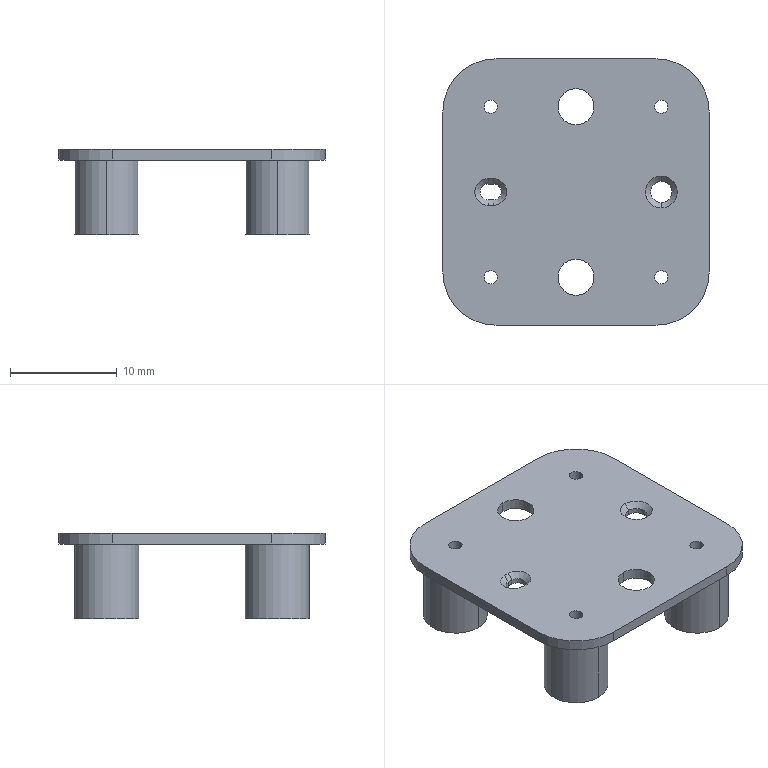NC program | NX | posted with a generic post | part box 25 x 25 x 8 mm
Whole program, first 1563 of 1707 lines:
N10 G17 G21 G94 G90
(FLOOR_WALL_COPY_COPY , TOOL : D80)
N12 T19 M6
N14 G54
N16 G17 G0 G90 X-57.5 Y0. S6500 M3
N18 G43 Z30. H19
N20 Z6.
N22 G94 G1 Z3. F1500.
N24 X-52.5
N26 X52.5
N28 X57.5
N30 Z6.
N32 G0 Z30.
N34 X-57.5
N36 Z5.
N38 G1 Z2.
N40 X-52.5
N42 X52.5
N44 X57.5
N46 Z5.
N48 G0 Z30.
N50 X-57.5
N52 Z4.
N54 G1 Z1.
N56 X-52.5
N58 X52.5
N60 X57.5
N62 Z4.
N64 G0 Z30.
N66 X-57.5
N68 Z3.
N70 G1 Z0.
N72 X-52.5
N74 X52.5
N76 X57.5
N78 Z3.
N80 G0 Z30.
N82 M5
(FLOOR_WALL , TOOL : D4)
N84 T11 M6
N86 G54
N88 G17 G0 G90 X1.026 Y-15.5 S9500 M3
N90 G43 Z30. H11
N92 Z0.617
N94 G94 G1 Z-0.383 F1000.
N96 X0.306 Y-14.643
N98 G3 X0. Y-14.5 R0.4
N100 G1 X-7.5 F2000.
N102 G2 X-14.5 Y-7.5 R7.
N104 G1 Y7.5
N106 G2 X-7.5 Y14.5 R7.
N108 G1 X7.5
N110 G2 X14.5 Y7.5 R7.
N112 G1 Y-7.5
N114 G2 X7.5 Y-14.5 R7.
N116 G1 X0.
N118 Y-12.5
N120 X-4.838
N122 G3 X-12.5 Y-4.838 R-5.5
N124 G1 X-12.173 Y-5.068
N126 G2 X-5.068 Y-3.827 R5.1
N128 X-12.173 Y-5.068 R-5.1
N130 G1 X-12.5 Y-4.838
N132 Y4.838
N134 G3 X-4.838 Y12.5 R-5.5
N136 G1 X-5.068 Y12.173
N138 G2 X-3.827 Y5.068 R5.1
N140 X-5.068 Y12.173 R-5.1
N142 G1 X-4.838 Y12.5
N144 X4.838
N146 G3 X12.5 Y4.838 R-5.5
N148 G1 X12.173 Y5.068
N150 G2 X5.068 Y3.827 R5.1
N152 X12.173 Y5.068 R-5.1
N154 G1 X12.5 Y4.838
N156 Y-4.838
N158 G3 X4.838 Y-12.5 R-5.5
N160 G1 X5.068 Y-12.173
N162 G2 X3.827 Y-5.068 R5.1
N164 X5.068 Y-12.173 R-5.1
N166 G1 X4.838 Y-12.5
N168 X0.
N170 Y-10.5
N172 X-0.929
N174 G3 X-10.5 Y-0.929 R7.5
N176 G1 Y0.929
N178 G3 X-0.929 Y10.5 R7.5
N180 G1 X0.929
N182 G3 X10.5 Y0.929 R7.5
N184 G1 Y-0.929
N186 G3 X1.684 Y-3.955 R7.5
N188 G1 X0. Y-2.877
N190 G3 X-2.877 Y0. R9.5
N192 X0. Y2.877 R9.5
N194 X2.877 Y0. R9.5
N196 X0. Y-2.877 R9.5
N198 G1 Y-0.019
N200 X-0.019 Y0.
N202 X0. Y0.019
N204 X0.019 Y0.
N206 X0. Y-0.019
N208 Y-2.877
N210 X1.684 Y-3.955
N212 G3 X0.929 Y-10.5 R7.5
N214 G1 X0.
N216 G3 X-0.306 Y-10.643 R0.4
N218 G1 Z0.617
N220 G0 X1.026 Y-15.5 Z0.233
N222 G1 Z-0.767 F1000.
N224 X0.306 Y-14.643
N226 G3 X0. Y-14.5 R0.4
N228 G1 X-7.5 F2000.
N230 G2 X-14.5 Y-7.5 R7.
N232 G1 Y7.5
N234 G2 X-7.5 Y14.5 R7.
N236 G1 X7.5
N238 G2 X14.5 Y7.5 R7.
N240 G1 Y-7.5
N242 G2 X7.5 Y-14.5 R7.
N244 G1 X0.
N246 Y-12.5
N248 X-4.838
N250 G3 X-12.5 Y-4.838 R-5.5
N252 G1 X-12.173 Y-5.068
N254 G2 X-5.068 Y-3.827 R5.1
N256 X-12.173 Y-5.068 R-5.1
N258 G1 X-12.5 Y-4.838
N260 Y4.838
N262 G3 X-4.838 Y12.5 R-5.5
N264 G1 X-5.068 Y12.173
N266 G2 X-3.827 Y5.068 R5.1
N268 X-5.068 Y12.173 R-5.1
N270 G1 X-4.838 Y12.5
N272 X4.838
N274 G3 X12.5 Y4.838 R-5.5
N276 G1 X12.173 Y5.068
N278 G2 X5.068 Y3.827 R5.1
N280 X12.173 Y5.068 R-5.1
N282 G1 X12.5 Y4.838
N284 Y-4.838
N286 G3 X4.838 Y-12.5 R-5.5
N288 G1 X5.068 Y-12.173
N290 G2 X3.827 Y-5.068 R5.1
N292 X5.068 Y-12.173 R-5.1
N294 G1 X4.838 Y-12.5
N296 X0.
N298 Y-10.5
N300 X-0.929
N302 G3 X-10.5 Y-0.929 R7.5
N304 G1 Y0.929
N306 G3 X-0.929 Y10.5 R7.5
N308 G1 X0.929
N310 G3 X10.5 Y0.929 R7.5
N312 G1 Y-0.929
N314 G3 X1.684 Y-3.955 R7.5
N316 G1 X0. Y-2.877
N318 G3 X-2.877 Y0. R9.5
N320 X0. Y2.877 R9.5
N322 X2.877 Y0. R9.5
N324 X0. Y-2.877 R9.5
N326 G1 Y-0.019
N328 X-0.019 Y0.
N330 X0. Y0.019
N332 X0.019 Y0.
N334 X0. Y-0.019
N336 Y-2.877
N338 X1.684 Y-3.955
N340 G3 X0.929 Y-10.5 R7.5
N342 G1 X0.
N344 G3 X-0.306 Y-10.643 R0.4
N346 G1 Z0.233
N348 G0 X1.026 Y-15.5 Z-0.15
N350 G1 Z-1.15 F1000.
N352 X0.306 Y-14.643
N354 G3 X0. Y-14.5 R0.4
N356 G1 X-7.5 F2000.
N358 G2 X-14.5 Y-7.5 R7.
N360 G1 Y7.5
N362 G2 X-7.5 Y14.5 R7.
N364 G1 X7.5
N366 G2 X14.5 Y7.5 R7.
N368 G1 Y-7.5
N370 G2 X7.5 Y-14.5 R7.
N372 G1 X0.
N374 Y-12.5
N376 X-4.838
N378 G3 X-12.5 Y-4.838 R-5.5
N380 G1 X-12.173 Y-5.068
N382 G2 X-5.068 Y-3.827 R5.1
N384 X-12.173 Y-5.068 R-5.1
N386 G1 X-12.5 Y-4.838
N388 Y4.838
N390 G3 X-4.838 Y12.5 R-5.5
N392 G1 X-5.068 Y12.173
N394 G2 X-3.827 Y5.068 R5.1
N396 X-5.068 Y12.173 R-5.1
N398 G1 X-4.838 Y12.5
N400 X4.838
N402 G3 X12.5 Y4.838 R-5.5
N404 G1 X12.173 Y5.068
N406 G2 X5.068 Y3.827 R5.1
N408 X12.173 Y5.068 R-5.1
N410 G1 X12.5 Y4.838
N412 Y-4.838
N414 G3 X4.838 Y-12.5 R-5.5
N416 G1 X5.068 Y-12.173
N418 G2 X3.827 Y-5.068 R5.1
N420 X5.068 Y-12.173 R-5.1
N422 G1 X4.838 Y-12.5
N424 X0.
N426 Y-10.5
N428 X-0.929
N430 G3 X-10.5 Y-0.929 R7.5
N432 G1 Y0.929
N434 G3 X-0.929 Y10.5 R7.5
N436 G1 X0.929
N438 G3 X10.5 Y0.929 R7.5
N440 G1 Y-0.929
N442 G3 X1.684 Y-3.955 R7.5
N444 G1 X0. Y-2.877
N446 G3 X-2.877 Y0. R9.5
N448 X0. Y2.877 R9.5
N450 X2.877 Y0. R9.5
N452 X0. Y-2.877 R9.5
N454 G1 Y-0.019
N456 X-0.019 Y0.
N458 X0. Y0.019
N460 X0.019 Y0.
N462 X0. Y-0.019
N464 Y-2.877
N466 X1.684 Y-3.955
N468 G3 X0.929 Y-10.5 R7.5
N470 G1 X0.
N472 G3 X-0.306 Y-10.643 R0.4
N474 G1 Z-0.15
N476 G0 X1.026 Y-15.5 Z-0.533
N478 G1 Z-1.533 F1000.
N480 X0.306 Y-14.643
N482 G3 X0. Y-14.5 R0.4
N484 G1 X-7.5 F2000.
N486 G2 X-14.5 Y-7.5 R7.
N488 G1 Y7.5
N490 G2 X-7.5 Y14.5 R7.
N492 G1 X7.5
N494 G2 X14.5 Y7.5 R7.
N496 G1 Y-7.5
N498 G2 X7.5 Y-14.5 R7.
N500 G1 X0.
N502 Y-12.5
N504 X-4.838
N506 G3 X-12.5 Y-4.838 R-5.5
N508 G1 X-12.173 Y-5.068
N510 G2 X-5.068 Y-3.827 R5.1
N512 X-12.173 Y-5.068 R-5.1
N514 G1 X-12.5 Y-4.838
N516 Y4.838
N518 G3 X-4.838 Y12.5 R-5.5
N520 G1 X-5.068 Y12.173
N522 G2 X-3.827 Y5.068 R5.1
N524 X-5.068 Y12.173 R-5.1
N526 G1 X-4.838 Y12.5
N528 X4.838
N530 G3 X12.5 Y4.838 R-5.5
N532 G1 X12.173 Y5.068
N534 G2 X5.068 Y3.827 R5.1
N536 X12.173 Y5.068 R-5.1
N538 G1 X12.5 Y4.838
N540 Y-4.838
N542 G3 X4.838 Y-12.5 R-5.5
N544 G1 X5.068 Y-12.173
N546 G2 X3.827 Y-5.068 R5.1
N548 X5.068 Y-12.173 R-5.1
N550 G1 X4.838 Y-12.5
N552 X0.
N554 Y-10.5
N556 X-0.929
N558 G3 X-10.5 Y-0.929 R7.5
N560 G1 Y0.929
N562 G3 X-0.929 Y10.5 R7.5
N564 G1 X0.929
N566 G3 X10.5 Y0.929 R7.5
N568 G1 Y-0.929
N570 G3 X1.684 Y-3.955 R7.5
N572 G1 X0. Y-2.877
N574 G3 X-2.877 Y0. R9.5
N576 X0. Y2.877 R9.5
N578 X2.877 Y0. R9.5
N580 X0. Y-2.877 R9.5
N582 G1 Y-0.019
N584 X-0.019 Y0.
N586 X0. Y0.019
N588 X0.019 Y0.
N590 X0. Y-0.019
N592 Y-2.877
N594 X1.684 Y-3.955
N596 G3 X0.929 Y-10.5 R7.5
N598 G1 X0.
N600 G3 X-0.306 Y-10.643 R0.4
N602 G1 Z-0.533
N604 G0 X1.026 Y-15.5 Z-0.917
N606 G1 Z-1.917 F1000.
N608 X0.306 Y-14.643
N610 G3 X0. Y-14.5 R0.4
N612 G1 X-7.5 F2000.
N614 G2 X-14.5 Y-7.5 R7.
N616 G1 Y7.5
N618 G2 X-7.5 Y14.5 R7.
N620 G1 X7.5
N622 G2 X14.5 Y7.5 R7.
N624 G1 Y-7.5
N626 G2 X7.5 Y-14.5 R7.
N628 G1 X0.
N630 Y-12.5
N632 X-4.838
N634 G3 X-12.5 Y-4.838 R-5.5
N636 G1 X-12.173 Y-5.068
N638 G2 X-5.068 Y-3.827 R5.1
N640 X-12.173 Y-5.068 R-5.1
N642 G1 X-12.5 Y-4.838
N644 Y4.838
N646 G3 X-4.838 Y12.5 R-5.5
N648 G1 X-5.068 Y12.173
N650 G2 X-3.827 Y5.068 R5.1
N652 X-5.068 Y12.173 R-5.1
N654 G1 X-4.838 Y12.5
N656 X4.838
N658 G3 X12.5 Y4.838 R-5.5
N660 G1 X12.173 Y5.068
N662 G2 X5.068 Y3.827 R5.1
N664 X12.173 Y5.068 R-5.1
N666 G1 X12.5 Y4.838
N668 Y-4.838
N670 G3 X4.838 Y-12.5 R-5.5
N672 G1 X5.068 Y-12.173
N674 G2 X3.827 Y-5.068 R5.1
N676 X5.068 Y-12.173 R-5.1
N678 G1 X4.838 Y-12.5
N680 X0.
N682 Y-10.5
N684 X-0.929
N686 G3 X-10.5 Y-0.929 R7.5
N688 G1 Y0.929
N690 G3 X-0.929 Y10.5 R7.5
N692 G1 X0.929
N694 G3 X10.5 Y0.929 R7.5
N696 G1 Y-0.929
N698 G3 X1.684 Y-3.955 R7.5
N700 G1 X0. Y-2.877
N702 G3 X-2.877 Y0. R9.5
N704 X0. Y2.877 R9.5
N706 X2.877 Y0. R9.5
N708 X0. Y-2.877 R9.5
N710 G1 Y-0.019
N712 X-0.019 Y0.
N714 X0. Y0.019
N716 X0.019 Y0.
N718 X0. Y-0.019
N720 Y-2.877
N722 X1.684 Y-3.955
N724 G3 X0.929 Y-10.5 R7.5
N726 G1 X0.
N728 G3 X-0.306 Y-10.643 R0.4
N730 G1 Z-0.917
N732 G0 X1.026 Y-15.5 Z-1.3
N734 G1 Z-2.3 F1000.
N736 X0.306 Y-14.643
N738 G3 X0. Y-14.5 R0.4
N740 G1 X-7.5 F2000.
N742 G2 X-14.5 Y-7.5 R7.
N744 G1 Y7.5
N746 G2 X-7.5 Y14.5 R7.
N748 G1 X7.5
N750 G2 X14.5 Y7.5 R7.
N752 G1 Y-7.5
N754 G2 X7.5 Y-14.5 R7.
N756 G1 X0.
N758 Y-12.5
N760 X-4.838
N762 G3 X-12.5 Y-4.838 R-5.5
N764 G1 X-12.173 Y-5.068
N766 G2 X-5.068 Y-3.827 R5.1
N768 X-12.173 Y-5.068 R-5.1
N770 G1 X-12.5 Y-4.838
N772 Y4.838
N774 G3 X-4.838 Y12.5 R-5.5
N776 G1 X-5.068 Y12.173
N778 G2 X-3.827 Y5.068 R5.1
N780 X-5.068 Y12.173 R-5.1
N782 G1 X-4.838 Y12.5
N784 X4.838
N786 G3 X12.5 Y4.838 R-5.5
N788 G1 X12.173 Y5.068
N790 G2 X5.068 Y3.827 R5.1
N792 X12.173 Y5.068 R-5.1
N794 G1 X12.5 Y4.838
N796 Y-4.838
N798 G3 X4.838 Y-12.5 R-5.5
N800 G1 X5.068 Y-12.173
N802 G2 X3.827 Y-5.068 R5.1
N804 X5.068 Y-12.173 R-5.1
N806 G1 X4.838 Y-12.5
N808 X0.
N810 Y-10.5
N812 X-0.929
N814 G3 X-10.5 Y-0.929 R7.5
N816 G1 Y0.929
N818 G3 X-0.929 Y10.5 R7.5
N820 G1 X0.929
N822 G3 X10.5 Y0.929 R7.5
N824 G1 Y-0.929
N826 G3 X1.684 Y-3.955 R7.5
N828 G1 X0. Y-2.877
N830 G3 X-2.877 Y0. R9.5
N832 X0. Y2.877 R9.5
N834 X2.877 Y0. R9.5
N836 X0. Y-2.877 R9.5
N838 G1 Y-0.019
N840 X-0.019 Y0.
N842 X0. Y0.019
N844 X0.019 Y0.
N846 X0. Y-0.019
N848 Y-2.877
N850 X1.684 Y-3.955
N852 G3 X0.929 Y-10.5 R7.5
N854 G1 X0.
N856 G3 X-0.306 Y-10.643 R0.4
N858 G1 Z-1.3
N860 G0 X1.026 Y-15.5 Z-1.683
N862 G1 Z-2.683 F1000.
N864 X0.306 Y-14.643
N866 G3 X0. Y-14.5 R0.4
N868 G1 X-7.5 F2000.
N870 G2 X-14.5 Y-7.5 R7.
N872 G1 Y7.5
N874 G2 X-7.5 Y14.5 R7.
N876 G1 X7.5
N878 G2 X14.5 Y7.5 R7.
N880 G1 Y-7.5
N882 G2 X7.5 Y-14.5 R7.
N884 G1 X0.
N886 Y-12.5
N888 X-4.838
N890 G3 X-12.5 Y-4.838 R-5.5
N892 G1 X-12.173 Y-5.068
N894 G2 X-5.068 Y-3.827 R5.1
N896 X-12.173 Y-5.068 R-5.1
N898 G1 X-12.5 Y-4.838
N900 Y4.838
N902 G3 X-4.838 Y12.5 R-5.5
N904 G1 X-5.068 Y12.173
N906 G2 X-3.827 Y5.068 R5.1
N908 X-5.068 Y12.173 R-5.1
N910 G1 X-4.838 Y12.5
N912 X4.838
N914 G3 X12.5 Y4.838 R-5.5
N916 G1 X12.173 Y5.068
N918 G2 X5.068 Y3.827 R5.1
N920 X12.173 Y5.068 R-5.1
N922 G1 X12.5 Y4.838
N924 Y-4.838
N926 G3 X4.838 Y-12.5 R-5.5
N928 G1 X5.068 Y-12.173
N930 G2 X3.827 Y-5.068 R5.1
N932 X5.068 Y-12.173 R-5.1
N934 G1 X4.838 Y-12.5
N936 X0.
N938 Y-10.5
N940 X-0.929
N942 G3 X-10.5 Y-0.929 R7.5
N944 G1 Y0.929
N946 G3 X-0.929 Y10.5 R7.5
N948 G1 X0.929
N950 G3 X10.5 Y0.929 R7.5
N952 G1 Y-0.929
N954 G3 X1.684 Y-3.955 R7.5
N956 G1 X0. Y-2.877
N958 G3 X-2.877 Y0. R9.5
N960 X0. Y2.877 R9.5
N962 X2.877 Y0. R9.5
N964 X0. Y-2.877 R9.5
N966 G1 Y-0.019
N968 X-0.019 Y0.
N970 X0. Y0.019
N972 X0.019 Y0.
N974 X0. Y-0.019
N976 Y-2.877
N978 X1.684 Y-3.955
N980 G3 X0.929 Y-10.5 R7.5
N982 G1 X0.
N984 G3 X-0.306 Y-10.643 R0.4
N986 G1 Z-1.683
N988 G0 X1.026 Y-15.5 Z-2.067
N990 G1 Z-3.067 F1000.
N992 X0.306 Y-14.643
N994 G3 X0. Y-14.5 R0.4
N996 G1 X-7.5 F2000.
N998 G2 X-14.5 Y-7.5 R7.
N1000 G1 Y7.5
N1002 G2 X-7.5 Y14.5 R7.
N1004 G1 X7.5
N1006 G2 X14.5 Y7.5 R7.
N1008 G1 Y-7.5
N1010 G2 X7.5 Y-14.5 R7.
N1012 G1 X0.
N1014 Y-12.5
N1016 X-4.838
N1018 G3 X-12.5 Y-4.838 R-5.5
N1020 G1 X-12.173 Y-5.068
N1022 G2 X-5.068 Y-3.827 R5.1
N1024 X-12.173 Y-5.068 R-5.1
N1026 G1 X-12.5 Y-4.838
N1028 Y4.838
N1030 G3 X-4.838 Y12.5 R-5.5
N1032 G1 X-5.068 Y12.173
N1034 G2 X-3.827 Y5.068 R5.1
N1036 X-5.068 Y12.173 R-5.1
N1038 G1 X-4.838 Y12.5
N1040 X4.838
N1042 G3 X12.5 Y4.838 R-5.5
N1044 G1 X12.173 Y5.068
N1046 G2 X5.068 Y3.827 R5.1
N1048 X12.173 Y5.068 R-5.1
N1050 G1 X12.5 Y4.838
N1052 Y-4.838
N1054 G3 X4.838 Y-12.5 R-5.5
N1056 G1 X5.068 Y-12.173
N1058 G2 X3.827 Y-5.068 R5.1
N1060 X5.068 Y-12.173 R-5.1
N1062 G1 X4.838 Y-12.5
N1064 X0.
N1066 Y-10.5
N1068 X-0.929
N1070 G3 X-10.5 Y-0.929 R7.5
N1072 G1 Y0.929
N1074 G3 X-0.929 Y10.5 R7.5
N1076 G1 X0.929
N1078 G3 X10.5 Y0.929 R7.5
N1080 G1 Y-0.929
N1082 G3 X1.684 Y-3.955 R7.5
N1084 G1 X0. Y-2.877
N1086 G3 X-2.877 Y0. R9.5
N1088 X0. Y2.877 R9.5
N1090 X2.877 Y0. R9.5
N1092 X0. Y-2.877 R9.5
N1094 G1 Y-0.019
N1096 X-0.019 Y0.
N1098 X0. Y0.019
N1100 X0.019 Y0.
N1102 X0. Y-0.019
N1104 Y-2.877
N1106 X1.684 Y-3.955
N1108 G3 X0.929 Y-10.5 R7.5
N1110 G1 X0.
N1112 G3 X-0.306 Y-10.643 R0.4
N1114 G1 Z-2.067
N1116 G0 X1.026 Y-15.5 Z-2.45
N1118 G1 Z-3.45 F1000.
N1120 X0.306 Y-14.643
N1122 G3 X0. Y-14.5 R0.4
N1124 G1 X-7.5 F2000.
N1126 G2 X-14.5 Y-7.5 R7.
N1128 G1 Y7.5
N1130 G2 X-7.5 Y14.5 R7.
N1132 G1 X7.5
N1134 G2 X14.5 Y7.5 R7.
N1136 G1 Y-7.5
N1138 G2 X7.5 Y-14.5 R7.
N1140 G1 X0.
N1142 Y-12.5
N1144 X-4.838
N1146 G3 X-12.5 Y-4.838 R-5.5
N1148 G1 X-12.173 Y-5.068
N1150 G2 X-5.068 Y-3.827 R5.1
N1152 X-12.173 Y-5.068 R-5.1
N1154 G1 X-12.5 Y-4.838
N1156 Y4.838
N1158 G3 X-4.838 Y12.5 R-5.5
N1160 G1 X-5.068 Y12.173
N1162 G2 X-3.827 Y5.068 R5.1
N1164 X-5.068 Y12.173 R-5.1
N1166 G1 X-4.838 Y12.5
N1168 X4.838
N1170 G3 X12.5 Y4.838 R-5.5
N1172 G1 X12.173 Y5.068
N1174 G2 X5.068 Y3.827 R5.1
N1176 X12.173 Y5.068 R-5.1
N1178 G1 X12.5 Y4.838
N1180 Y-4.838
N1182 G3 X4.838 Y-12.5 R-5.5
N1184 G1 X5.068 Y-12.173
N1186 G2 X3.827 Y-5.068 R5.1
N1188 X5.068 Y-12.173 R-5.1
N1190 G1 X4.838 Y-12.5
N1192 X0.
N1194 Y-10.5
N1196 X-0.929
N1198 G3 X-10.5 Y-0.929 R7.5
N1200 G1 Y0.929
N1202 G3 X-0.929 Y10.5 R7.5
N1204 G1 X0.929
N1206 G3 X10.5 Y0.929 R7.5
N1208 G1 Y-0.929
N1210 G3 X1.684 Y-3.955 R7.5
N1212 G1 X0. Y-2.877
N1214 G3 X-2.877 Y0. R9.5
N1216 X0. Y2.877 R9.5
N1218 X2.877 Y0. R9.5
N1220 X0. Y-2.877 R9.5
N1222 G1 Y-0.019
N1224 X-0.019 Y0.
N1226 X0. Y0.019
N1228 X0.019 Y0.
N1230 X0. Y-0.019
N1232 Y-2.877
N1234 X1.684 Y-3.955
N1236 G3 X0.929 Y-10.5 R7.5
N1238 G1 X0.
N1240 G3 X-0.306 Y-10.643 R0.4
N1242 G1 Z-2.45
N1244 G0 X1.026 Y-15.5 Z-2.833
N1246 G1 Z-3.833 F1000.
N1248 X0.306 Y-14.643
N1250 G3 X0. Y-14.5 R0.4
N1252 G1 X-7.5 F2000.
N1254 G2 X-14.5 Y-7.5 R7.
N1256 G1 Y7.5
N1258 G2 X-7.5 Y14.5 R7.
N1260 G1 X7.5
N1262 G2 X14.5 Y7.5 R7.
N1264 G1 Y-7.5
N1266 G2 X7.5 Y-14.5 R7.
N1268 G1 X0.
N1270 Y-12.5
N1272 X-4.838
N1274 G3 X-12.5 Y-4.838 R-5.5
N1276 G1 X-12.173 Y-5.068
N1278 G2 X-5.068 Y-3.827 R5.1
N1280 X-12.173 Y-5.068 R-5.1
N1282 G1 X-12.5 Y-4.838
N1284 Y4.838
N1286 G3 X-4.838 Y12.5 R-5.5
N1288 G1 X-5.068 Y12.173
N1290 G2 X-3.827 Y5.068 R5.1
N1292 X-5.068 Y12.173 R-5.1
N1294 G1 X-4.838 Y12.5
N1296 X4.838
N1298 G3 X12.5 Y4.838 R-5.5
N1300 G1 X12.173 Y5.068
N1302 G2 X5.068 Y3.827 R5.1
N1304 X12.173 Y5.068 R-5.1
N1306 G1 X12.5 Y4.838
N1308 Y-4.838
N1310 G3 X4.838 Y-12.5 R-5.5
N1312 G1 X5.068 Y-12.173
N1314 G2 X3.827 Y-5.068 R5.1
N1316 X5.068 Y-12.173 R-5.1
N1318 G1 X4.838 Y-12.5
N1320 X0.
N1322 Y-10.5
N1324 X-0.929
N1326 G3 X-10.5 Y-0.929 R7.5
N1328 G1 Y0.929
N1330 G3 X-0.929 Y10.5 R7.5
N1332 G1 X0.929
N1334 G3 X10.5 Y0.929 R7.5
N1336 G1 Y-0.929
N1338 G3 X1.684 Y-3.955 R7.5
N1340 G1 X0. Y-2.877
N1342 G3 X-2.877 Y0. R9.5
N1344 X0. Y2.877 R9.5
N1346 X2.877 Y0. R9.5
N1348 X0. Y-2.877 R9.5
N1350 G1 Y-0.019
N1352 X-0.019 Y0.
N1354 X0. Y0.019
N1356 X0.019 Y0.
N1358 X0. Y-0.019
N1360 Y-2.877
N1362 X1.684 Y-3.955
N1364 G3 X0.929 Y-10.5 R7.5
N1366 G1 X0.
N1368 G3 X-0.306 Y-10.643 R0.4
N1370 G1 Z-2.833
N1372 G0 X1.026 Y-15.5 Z-3.217
N1374 G1 Z-4.217 F1000.
N1376 X0.306 Y-14.643
N1378 G3 X0. Y-14.5 R0.4
N1380 G1 X-7.5 F2000.
N1382 G2 X-14.5 Y-7.5 R7.
N1384 G1 Y7.5
N1386 G2 X-7.5 Y14.5 R7.
N1388 G1 X7.5
N1390 G2 X14.5 Y7.5 R7.
N1392 G1 Y-7.5
N1394 G2 X7.5 Y-14.5 R7.
N1396 G1 X0.
N1398 Y-12.5
N1400 X-4.838
N1402 G3 X-12.5 Y-4.838 R-5.5
N1404 G1 X-12.173 Y-5.068
N1406 G2 X-5.068 Y-3.827 R5.1
N1408 X-12.173 Y-5.068 R-5.1
N1410 G1 X-12.5 Y-4.838
N1412 Y4.838
N1414 G3 X-4.838 Y12.5 R-5.5
N1416 G1 X-5.068 Y12.173
N1418 G2 X-3.827 Y5.068 R5.1
N1420 X-5.068 Y12.173 R-5.1
N1422 G1 X-4.838 Y12.5
N1424 X4.838
N1426 G3 X12.5 Y4.838 R-5.5
N1428 G1 X12.173 Y5.068
N1430 G2 X5.068 Y3.827 R5.1
N1432 X12.173 Y5.068 R-5.1
N1434 G1 X12.5 Y4.838
N1436 Y-4.838
N1438 G3 X4.838 Y-12.5 R-5.5
N1440 G1 X5.068 Y-12.173
N1442 G2 X3.827 Y-5.068 R5.1
N1444 X5.068 Y-12.173 R-5.1
N1446 G1 X4.838 Y-12.5
N1448 X0.
N1450 Y-10.5
N1452 X-0.929
N1454 G3 X-10.5 Y-0.929 R7.5
N1456 G1 Y0.929
N1458 G3 X-0.929 Y10.5 R7.5
N1460 G1 X0.929
N1462 G3 X10.5 Y0.929 R7.5
N1464 G1 Y-0.929
N1466 G3 X1.684 Y-3.955 R7.5
N1468 G1 X0. Y-2.877
N1470 G3 X-2.877 Y0. R9.5
N1472 X0. Y2.877 R9.5
N1474 X2.877 Y0. R9.5
N1476 X0. Y-2.877 R9.5
N1478 G1 Y-0.019
N1480 X-0.019 Y0.
N1482 X0. Y0.019
N1484 X0.019 Y0.
N1486 X0. Y-0.019
N1488 Y-2.877
N1490 X1.684 Y-3.955
N1492 G3 X0.929 Y-10.5 R7.5
N1494 G1 X0.
N1496 G3 X-0.306 Y-10.643 R0.4
N1498 G1 Z-3.217
N1500 G0 X1.026 Y-15.5 Z-3.6
N1502 G1 Z-4.6 F1000.
N1504 X0.306 Y-14.643
N1506 G3 X0. Y-14.5 R0.4
N1508 G1 X-7.5 F2000.
N1510 G2 X-14.5 Y-7.5 R7.
N1512 G1 Y7.5
N1514 G2 X-7.5 Y14.5 R7.
N1516 G1 X7.5
N1518 G2 X14.5 Y7.5 R7.
N1520 G1 Y-7.5
N1522 G2 X7.5 Y-14.5 R7.
N1524 G1 X0.
N1526 Y-12.5
N1528 X-4.838
N1530 G3 X-12.5 Y-4.838 R-5.5
N1532 G1 X-12.173 Y-5.068
N1534 G2 X-5.068 Y-3.827 R5.1
N1536 X-12.173 Y-5.068 R-5.1
N1538 G1 X-12.5 Y-4.838
N1540 Y4.838
N1542 G3 X-4.838 Y12.5 R-5.5
N1544 G1 X-5.068 Y12.173
N1546 G2 X-3.827 Y5.068 R5.1
N1548 X-5.068 Y12.173 R-5.1
N1550 G1 X-4.838 Y12.5
N1552 X4.838
N1554 G3 X12.5 Y4.838 R-5.5
N1556 G1 X12.173 Y5.068
N1558 G2 X5.068 Y3.827 R5.1
N1560 X12.173 Y5.068 R-5.1
N1562 G1 X12.5 Y4.838
N1564 Y-4.838
N1566 G3 X4.838 Y-12.5 R-5.5
N1568 G1 X5.068 Y-12.173
N1570 G2 X3.827 Y-5.068 R5.1
N1572 X5.068 Y-12.173 R-5.1
N1574 G1 X4.838 Y-12.5
N1576 X0.
N1578 Y-10.5
N1580 X-0.929
N1582 G3 X-10.5 Y-0.929 R7.5
N1584 G1 Y0.929
N1586 G3 X-0.929 Y10.5 R7.5
N1588 G1 X0.929
N1590 G3 X10.5 Y0.929 R7.5
N1592 G1 Y-0.929
N1594 G3 X1.684 Y-3.955 R7.5
N1596 G1 X0. Y-2.877
N1598 G3 X-2.877 Y0. R9.5
N1600 X0. Y2.877 R9.5
N1602 X2.877 Y0. R9.5
N1604 X0. Y-2.877 R9.5
N1606 G1 Y-0.019
N1608 X-0.019 Y0.
N1610 X0. Y0.019
N1612 X0.019 Y0.
N1614 X0. Y-0.019
N1616 Y-2.877
N1618 X1.684 Y-3.955
N1620 G3 X0.929 Y-10.5 R7.5
N1622 G1 X0.
N1624 G3 X-0.306 Y-10.643 R0.4
N1626 G1 Z-3.6
N1628 G0 X1.026 Y-15.5 Z-3.983
N1630 G1 Z-4.983 F1000.
N1632 X0.306 Y-14.643
N1634 G3 X0. Y-14.5 R0.4
N1636 G1 X-7.5 F2000.
N1638 G2 X-14.5 Y-7.5 R7.
N1640 G1 Y7.5
N1642 G2 X-7.5 Y14.5 R7.
N1644 G1 X7.5
N1646 G2 X14.5 Y7.5 R7.
N1648 G1 Y-7.5
N1650 G2 X7.5 Y-14.5 R7.
N1652 G1 X0.
N1654 Y-12.5
N1656 X-4.838
N1658 G3 X-12.5 Y-4.838 R-5.5
N1660 G1 X-12.173 Y-5.068
N1662 G2 X-5.068 Y-3.827 R5.1
N1664 X-12.173 Y-5.068 R-5.1
N1666 G1 X-12.5 Y-4.838
N1668 Y4.838
N1670 G3 X-4.838 Y12.5 R-5.5
N1672 G1 X-5.068 Y12.173
N1674 G2 X-3.827 Y5.068 R5.1
N1676 X-5.068 Y12.173 R-5.1
N1678 G1 X-4.838 Y12.5
N1680 X4.838
N1682 G3 X12.5 Y4.838 R-5.5
N1684 G1 X12.173 Y5.068
N1686 G2 X5.068 Y3.827 R5.1
N1688 X12.173 Y5.068 R-5.1
N1690 G1 X12.5 Y4.838
N1692 Y-4.838
N1694 G3 X4.838 Y-12.5 R-5.5
N1696 G1 X5.068 Y-12.173
N1698 G2 X3.827 Y-5.068 R5.1
N1700 X5.068 Y-12.173 R-5.1
N1702 G1 X4.838 Y-12.5
N1704 X0.
N1706 Y-10.5
N1708 X-0.929
N1710 G3 X-10.5 Y-0.929 R7.5
N1712 G1 Y0.929
N1714 G3 X-0.929 Y10.5 R7.5
N1716 G1 X0.929
N1718 G3 X10.5 Y0.929 R7.5
N1720 G1 Y-0.929
N1722 G3 X1.684 Y-3.955 R7.5
N1724 G1 X0. Y-2.877
N1726 G3 X-2.877 Y0. R9.5
N1728 X0. Y2.877 R9.5
N1730 X2.877 Y0. R9.5
N1732 X0. Y-2.877 R9.5
N1734 G1 Y-0.019
N1736 X-0.019 Y0.
N1738 X0. Y0.019
N1740 X0.019 Y0.
N1742 X0. Y-0.019
N1744 Y-2.877
N1746 X1.684 Y-3.955
N1748 G3 X0.929 Y-10.5 R7.5
N1750 G1 X0.
N1752 G3 X-0.306 Y-10.643 R0.4
N1754 G1 Z-3.983
N1756 G0 X1.026 Y-15.5 Z-4.367
N1758 G1 Z-5.367 F1000.
N1760 X0.306 Y-14.643
N1762 G3 X0. Y-14.5 R0.4
N1764 G1 X-7.5 F2000.
N1766 G2 X-14.5 Y-7.5 R7.
N1768 G1 Y7.5
N1770 G2 X-7.5 Y14.5 R7.
N1772 G1 X7.5
N1774 G2 X14.5 Y7.5 R7.
N1776 G1 Y-7.5
N1778 G2 X7.5 Y-14.5 R7.
N1780 G1 X0.
N1782 Y-12.5
N1784 X-4.838
N1786 G3 X-12.5 Y-4.838 R-5.5
N1788 G1 X-12.173 Y-5.068
N1790 G2 X-5.068 Y-3.827 R5.1
N1792 X-12.173 Y-5.068 R-5.1
N1794 G1 X-12.5 Y-4.838
N1796 Y4.838
N1798 G3 X-4.838 Y12.5 R-5.5
N1800 G1 X-5.068 Y12.173
N1802 G2 X-3.827 Y5.068 R5.1
N1804 X-5.068 Y12.173 R-5.1
N1806 G1 X-4.838 Y12.5
N1808 X4.838
N1810 G3 X12.5 Y4.838 R-5.5
N1812 G1 X12.173 Y5.068
N1814 G2 X5.068 Y3.827 R5.1
N1816 X12.173 Y5.068 R-5.1
N1818 G1 X12.5 Y4.838
N1820 Y-4.838
N1822 G3 X4.838 Y-12.5 R-5.5
N1824 G1 X5.068 Y-12.173
N1826 G2 X3.827 Y-5.068 R5.1
N1828 X5.068 Y-12.173 R-5.1
N1830 G1 X4.838 Y-12.5
N1832 X0.
N1834 Y-10.5
N1836 X-0.929
N1838 G3 X-10.5 Y-0.929 R7.5
N1840 G1 Y0.929
N1842 G3 X-0.929 Y10.5 R7.5
N1844 G1 X0.929
N1846 G3 X10.5 Y0.929 R7.5
N1848 G1 Y-0.929
N1850 G3 X1.684 Y-3.955 R7.5
N1852 G1 X0. Y-2.877
N1854 G3 X-2.877 Y0. R9.5
N1856 X0. Y2.877 R9.5
N1858 X2.877 Y0. R9.5
N1860 X0. Y-2.877 R9.5
N1862 G1 Y-0.019
N1864 X-0.019 Y0.
N1866 X0. Y0.019
N1868 X0.019 Y0.
N1870 X0. Y-0.019
N1872 Y-2.877
N1874 X1.684 Y-3.955
N1876 G3 X0.929 Y-10.5 R7.5
N1878 G1 X0.
N1880 G3 X-0.306 Y-10.643 R0.4
N1882 G1 Z-4.367
N1884 G0 X1.026 Y-15.5 Z-4.75
N1886 G1 Z-5.75 F1000.
N1888 X0.306 Y-14.643
N1890 G3 X0. Y-14.5 R0.4
N1892 G1 X-7.5 F2000.
N1894 G2 X-14.5 Y-7.5 R7.
N1896 G1 Y7.5
N1898 G2 X-7.5 Y14.5 R7.
N1900 G1 X7.5
N1902 G2 X14.5 Y7.5 R7.
N1904 G1 Y-7.5
N1906 G2 X7.5 Y-14.5 R7.
N1908 G1 X0.
N1910 Y-12.5
N1912 X-4.838
N1914 G3 X-12.5 Y-4.838 R-5.5
N1916 G1 X-12.173 Y-5.068
N1918 G2 X-5.068 Y-3.827 R5.1
N1920 X-12.173 Y-5.068 R-5.1
N1922 G1 X-12.5 Y-4.838
N1924 Y4.838
N1926 G3 X-4.838 Y12.5 R-5.5
N1928 G1 X-5.068 Y12.173
N1930 G2 X-3.827 Y5.068 R5.1
N1932 X-5.068 Y12.173 R-5.1
N1934 G1 X-4.838 Y12.5
N1936 X4.838
N1938 G3 X12.5 Y4.838 R-5.5
N1940 G1 X12.173 Y5.068
N1942 G2 X5.068 Y3.827 R5.1
N1944 X12.173 Y5.068 R-5.1
N1946 G1 X12.5 Y4.838
N1948 Y-4.838
N1950 G3 X4.838 Y-12.5 R-5.5
N1952 G1 X5.068 Y-12.173
N1954 G2 X3.827 Y-5.068 R5.1
N1956 X5.068 Y-12.173 R-5.1
N1958 G1 X4.838 Y-12.5
N1960 X0.
N1962 Y-10.5
N1964 X-0.929
N1966 G3 X-10.5 Y-0.929 R7.5
N1968 G1 Y0.929
N1970 G3 X-0.929 Y10.5 R7.5
N1972 G1 X0.929
N1974 G3 X10.5 Y0.929 R7.5
N1976 G1 Y-0.929
N1978 G3 X1.684 Y-3.955 R7.5
N1980 G1 X0. Y-2.877
N1982 G3 X-2.877 Y0. R9.5
N1984 X0. Y2.877 R9.5
N1986 X2.877 Y0. R9.5
N1988 X0. Y-2.877 R9.5
N1990 G1 Y-0.019
N1992 X-0.019 Y0.
N1994 X0. Y0.019
N1996 X0.019 Y0.
N1998 X0. Y-0.019
N2000 Y-2.877
N2002 X1.684 Y-3.955
N2004 G3 X0.929 Y-10.5 R7.5
N2006 G1 X0.
N2008 G3 X-0.306 Y-10.643 R0.4
N2010 G1 Z-4.75
N2012 G0 X1.026 Y-15.5 Z-5.133
N2014 G1 Z-6.133 F1000.
N2016 X0.306 Y-14.643
N2018 G3 X0. Y-14.5 R0.4
N2020 G1 X-7.5 F2000.
N2022 G2 X-14.5 Y-7.5 R7.
N2024 G1 Y7.5
N2026 G2 X-7.5 Y14.5 R7.
N2028 G1 X7.5
N2030 G2 X14.5 Y7.5 R7.
N2032 G1 Y-7.5
N2034 G2 X7.5 Y-14.5 R7.
N2036 G1 X0.
N2038 Y-12.5
N2040 X-4.838
N2042 G3 X-12.5 Y-4.838 R-5.5
N2044 G1 X-12.173 Y-5.068
N2046 G2 X-5.068 Y-3.827 R5.1
N2048 X-12.173 Y-5.068 R-5.1
N2050 G1 X-12.5 Y-4.838
N2052 Y4.838
N2054 G3 X-4.838 Y12.5 R-5.5
N2056 G1 X-5.068 Y12.173
N2058 G2 X-3.827 Y5.068 R5.1
N2060 X-5.068 Y12.173 R-5.1
N2062 G1 X-4.838 Y12.5
N2064 X4.838
N2066 G3 X12.5 Y4.838 R-5.5
N2068 G1 X12.173 Y5.068
N2070 G2 X5.068 Y3.827 R5.1
N2072 X12.173 Y5.068 R-5.1
N2074 G1 X12.5 Y4.838
N2076 Y-4.838
N2078 G3 X4.838 Y-12.5 R-5.5
N2080 G1 X5.068 Y-12.173
N2082 G2 X3.827 Y-5.068 R5.1
N2084 X5.068 Y-12.173 R-5.1
N2086 G1 X4.838 Y-12.5
N2088 X0.
N2090 Y-10.5
N2092 X-0.929
N2094 G3 X-10.5 Y-0.929 R7.5
N2096 G1 Y0.929
N2098 G3 X-0.929 Y10.5 R7.5
N2100 G1 X0.929
N2102 G3 X10.5 Y0.929 R7.5
N2104 G1 Y-0.929
N2106 G3 X1.684 Y-3.955 R7.5
N2108 G1 X0. Y-2.877
N2110 G3 X-2.877 Y0. R9.5
N2112 X0. Y2.877 R9.5
N2114 X2.877 Y0. R9.5
N2116 X0. Y-2.877 R9.5
N2118 G1 Y-0.019
N2120 X-0.019 Y0.
N2122 X0. Y0.019
N2124 X0.019 Y0.
N2126 X0. Y-0.019
N2128 Y-2.877
N2130 X1.684 Y-3.955
N2132 G3 X0.929 Y-10.5 R7.5
N2134 G1 X0.
N2136 G3 X-0.306 Y-10.643 R0.4
N2138 G1 Z-5.133
N2140 G0 X1.026 Y-15.5 Z-5.517
N2142 G1 Z-6.517 F1000.
N2144 X0.306 Y-14.643
N2146 G3 X0. Y-14.5 R0.4
N2148 G1 X-7.5 F2000.
N2150 G2 X-14.5 Y-7.5 R7.
N2152 G1 Y7.5
N2154 G2 X-7.5 Y14.5 R7.
N2156 G1 X7.5
N2158 G2 X14.5 Y7.5 R7.
N2160 G1 Y-7.5
N2162 G2 X7.5 Y-14.5 R7.
N2164 G1 X0.
N2166 Y-12.5
N2168 X-4.838
N2170 G3 X-12.5 Y-4.838 R-5.5
N2172 G1 X-12.173 Y-5.068
N2174 G2 X-5.068 Y-3.827 R5.1
N2176 X-12.173 Y-5.068 R-5.1
N2178 G1 X-12.5 Y-4.838
N2180 Y4.838
N2182 G3 X-4.838 Y12.5 R-5.5
N2184 G1 X-5.068 Y12.173
N2186 G2 X-3.827 Y5.068 R5.1
N2188 X-5.068 Y12.173 R-5.1
N2190 G1 X-4.838 Y12.5
N2192 X4.838
N2194 G3 X12.5 Y4.838 R-5.5
N2196 G1 X12.173 Y5.068
N2198 G2 X5.068 Y3.827 R5.1
N2200 X12.173 Y5.068 R-5.1
N2202 G1 X12.5 Y4.838
N2204 Y-4.838
N2206 G3 X4.838 Y-12.5 R-5.5
N2208 G1 X5.068 Y-12.173
N2210 G2 X3.827 Y-5.068 R5.1
N2212 X5.068 Y-12.173 R-5.1
N2214 G1 X4.838 Y-12.5
N2216 X0.
N2218 Y-10.5
N2220 X-0.929
N2222 G3 X-10.5 Y-0.929 R7.5
N2224 G1 Y0.929
N2226 G3 X-0.929 Y10.5 R7.5
N2228 G1 X0.929
N2230 G3 X10.5 Y0.929 R7.5
N2232 G1 Y-0.929
N2234 G3 X1.684 Y-3.955 R7.5
N2236 G1 X0. Y-2.877
N2238 G3 X-2.877 Y0. R9.5
N2240 X0. Y2.877 R9.5
N2242 X2.877 Y0. R9.5
N2244 X0. Y-2.877 R9.5
N2246 G1 Y-0.019
N2248 X-0.019 Y0.
N2250 X0. Y0.019
N2252 X0.019 Y0.
N2254 X0. Y-0.019
N2256 Y-2.877
N2258 X1.684 Y-3.955
N2260 G3 X0.929 Y-10.5 R7.5
N2262 G1 X0.
N2264 G3 X-0.306 Y-10.643 R0.4
N2266 G1 Z-5.517
N2268 G0 X1.026 Y-15.5 Z-5.9
N2270 G1 Z-6.9 F1000.
N2272 X0.306 Y-14.643
N2274 G3 X0. Y-14.5 R0.4
N2276 G1 X-7.5 F2000.
N2278 G2 X-14.5 Y-7.5 R7.
N2280 G1 Y7.5
N2282 G2 X-7.5 Y14.5 R7.
N2284 G1 X7.5
N2286 G2 X14.5 Y7.5 R7.
N2288 G1 Y-7.5
N2290 G2 X7.5 Y-14.5 R7.
N2292 G1 X0.
N2294 Y-12.5
N2296 X-4.838
N2298 G3 X-12.5 Y-4.838 R-5.5
N2300 G1 X-12.173 Y-5.068
N2302 G2 X-5.068 Y-3.827 R5.1
N2304 X-12.173 Y-5.068 R-5.1
N2306 G1 X-12.5 Y-4.838
N2308 Y4.838
N2310 G3 X-4.838 Y12.5 R-5.5
N2312 G1 X-5.068 Y12.173
N2314 G2 X-3.827 Y5.068 R5.1
N2316 X-5.068 Y12.173 R-5.1
N2318 G1 X-4.838 Y12.5
N2320 X4.838
N2322 G3 X12.5 Y4.838 R-5.5
N2324 G1 X12.173 Y5.068
N2326 G2 X5.068 Y3.827 R5.1
N2328 X12.173 Y5.068 R-5.1
N2330 G1 X12.5 Y4.838
N2332 Y-4.838
N2334 G3 X4.838 Y-12.5 R-5.5
N2336 G1 X5.068 Y-12.173
N2338 G2 X3.827 Y-5.068 R5.1
N2340 X5.068 Y-12.173 R-5.1
N2342 G1 X4.838 Y-12.5
N2344 X0.
N2346 Y-10.5
N2348 X-0.929
N2350 G3 X-10.5 Y-0.929 R7.5
N2352 G1 Y0.929
N2354 G3 X-0.929 Y10.5 R7.5
N2356 G1 X0.929
N2358 G3 X10.5 Y0.929 R7.5
N2360 G1 Y-0.929
N2362 G3 X1.684 Y-3.955 R7.5
N2364 G1 X0. Y-2.877
N2366 G3 X-2.877 Y0. R9.5
N2368 X0. Y2.877 R9.5
N2370 X2.877 Y0. R9.5
N2372 X0. Y-2.877 R9.5
N2374 G1 Y-0.019
N2376 X-0.019 Y0.
N2378 X0. Y0.019
N2380 X0.019 Y0.
N2382 X0. Y-0.019
N2384 Y-2.877
N2386 X1.684 Y-3.955
N2388 G3 X0.929 Y-10.5 R7.5
N2390 G1 X0.
N2392 G3 X-0.306 Y-10.643 R0.4
N2394 G1 Z-5.9
N2396 G0 Z30.
(FLOOR_WALL_COPY_1 , TOOL : D4)
N2398 X-7.886 Y14.69
N2400 Z-6.
N2402 G1 Z-7. F1100.
N2404 X-7.847 Y14.643
N2406 G3 X-7.541 Y14.5 R0.4
N2408 G1 X-5.329
N2410 X7.5
N2412 G2 X12.35 Y12.547 R7.
N2414 G1 X10.523
N2416 G2 X12.507 Y10.593 R5.2
N2418 G1 X13.779
N2420 G2 X14.407 Y8.639 R7.
N2422 G1 X13.161
N2424 G2 X13.031 Y6.685 R5.2
N2426 G1 X14.5 Y6.686
N2428 Y4.732
N2430 X12.044 Y4.731
N2432 Z-6.
N2434 G0 Z30.
N2436 X-10.976 Y12.546
N2438 Z-5.9
N2440 G1 X-10.525 Z-6.021
N2442 X-12.352 Z-6.51
N2444 X-10.525 Z-7.
N2446 X-12.352
N2448 G3 X-13.78 Y10.592 R7.
N2450 G1 X-12.508
N2452 G3 X-13.161 Y8.638 R5.2
N2454 G1 X-14.407
N2456 G3 X-14.5 Y7.5 R7.
N2458 G1 Y6.684
N2460 X-13.031
N2462 G3 X-12.043 Y4.73 R5.2
N2464 G1 X-14.5
N2466 G2 X-14.806 Y4.873 R0.4
N2468 G1 Z-6.
N2470 G0 Z30.
N2472 X10.523 Y12.547
N2474 Z-6.
N2476 G1 Z-7.
N2478 G3 X5.477 Y12.547 R5.2
N2480 G1 X-5.476 Y12.546
N2482 G2 X-3.492 Y10.592 R5.2
N2484 G1 X3.492 Y10.593
N2486 G3 X2.839 Y8.639 R5.2
N2488 G1 X-2.839 Y8.638
N2490 G2 X-2.969 Y6.685 R5.2
N2492 G1 X2.969
N2494 G3 X3.956 Y4.731 R5.2
N2496 G1 X-3.956
N2498 Z-6.
N2500 G0 Z30.
N2502 X-14.806 Y2.919
N2504 Z-6.
N2506 G1 Z-7.
N2508 G3 X-14.5 Y2.776 R0.4
N2510 G1 X14.5 Y2.778
N2512 Y0.824
N2514 X-14.5 Y0.822
N2516 Y-1.132
N2518 X14.5 Y-1.13
N2520 Y-3.084
N2522 X9.696
N2524 G2 X12.274 Y-5.038 R5.2
N2526 G1 X14.5
N2528 Y-6.992
N2530 X13.101
N2532 G2 X13.113 Y-8.946 R5.2
N2534 G1 X14.349
N2536 G2 X13.619 Y-10.9 R7.
N2538 G1 X12.317
N2540 G2 X9.866 Y-12.854 R5.2
N2542 G1 X12.01
N2544 G3 X12.316 Y-12.711 R0.4
N2546 G1 X12.387 Y-12.787
N2548 Z-6.
N2550 G0 Z30.
N2552 X-13.804 Y-3.085
N2554 Z-5.9
N2556 G1 X-9.699 Z-7.
N2558 X-14.5 Y-3.086
N2560 Y-5.039
N2562 X-12.275
N2564 G3 X-13.102 Y-6.993 R5.2
N2566 G1 X-14.5
N2568 Y-7.5
N2570 G3 X-14.349 Y-8.947 R7.
N2572 G1 X-13.113
N2574 G3 X-12.316 Y-10.901 R5.2
N2576 G1 X-13.618
N2578 G3 X-12.008 Y-12.855 R7.
N2580 G1 X-9.863
N2582 G3 X-10.2 Y-12.882 R0.4
N2584 G1 Z-6.
N2586 G0 Z30.
N2588 X9.696 Y-3.084
N2590 Z-6.
N2592 G1 Z-7.
N2594 G3 X6.304 Y-3.084 R5.2
N2596 G1 X-6.302 Y-3.085
N2598 G2 X-3.725 Y-5.039 R5.2
N2600 G1 X3.726 Y-5.038
N2602 G3 X2.899 Y-6.992 R5.2
N2604 G1 X-2.899 Y-6.993
N2606 G2 X-2.887 Y-8.947 R5.2
N2608 G1 X2.887 Y-8.946
N2610 G3 X3.684 Y-10.9 R5.2
N2612 G1 X-3.684
N2614 G2 X-6.136 Y-12.855 R5.2
N2616 G1 X6.134 Y-12.854
N2618 G3 X5.797 Y-12.881 R0.4
N2620 G1 X6.441 Y-12.91
N2622 G3 X6.206 Y-12.667 R0.4
N2624 G2 X3.333 Y-6.206 R5.
N2626 X6.206 Y-12.667 R-5.
N2628 G3 X5.869 Y-12.691 R0.4
N2630 G1 X5.602 Y-12.838
N2632 Z-6.
N2634 G0 Z30.
N2636 X-7.497 Y-13.377
N2638 Z-6.
N2640 G1 Z-7.
N2642 X-7.694 Y-13.143
N2644 G3 X-8. Y-13. R0.4
N2646 G2 X-13. Y-8. R5.
N2648 X-8. Y-13. R-5.
N2650 G3 X-8.306 Y-13.143 R0.4
N2652 G1 X-8.503 Y-13.377
N2654 Z-6.
N2656 G0 Z30.
N2658 X13.377 Y8.503
N2660 Z-6.
N2662 G1 Z-7.
N2664 X13.143 Y8.306
N2666 G3 X13. Y8. R0.4
N2668 G2 X8. Y3. R5.
N2670 X13. Y8. R-5.
N2672 G3 X13.143 Y7.694 R0.4
N2674 G1 X13.377 Y7.497
N2676 Z-6.
N2678 G0 Z30.
N2680 X-8.503 Y13.377
N2682 Z-6.
N2684 G1 Z-7.
N2686 X-8.306 Y13.143
N2688 G3 X-8. Y13. R0.4
N2690 G2 X-3. Y8. R5.
N2692 X-8. Y13. R-5.
N2694 G3 X-7.694 Y13.143 R0.4
N2696 G1 X-7.497 Y13.377
N2698 Z-6.
N2700 G0 Z30.
N2702 M5
(HOLE_MILLING , TOOL : D1.0)
N2704 T18 M6
N2706 G54
N2708 G17 G0 G90 X-8. Y8. S9500 M3
N2710 G43 Z30. H18
N2712 Z0.5
N2714 G94 G3 X-8.15 Y8.15 R0.15 F800.
N2716 X-8.3 Y8. R0.15
N2718 X-8.3 Y8. Z0.42 I0.3 J0.
N2720 X-8.3 Y8. Z0.34 I0.3 J0.
N2722 X-8.3 Y8. Z0.26 I0.3 J0.
N2724 X-8.3 Y8. Z0.18 I0.3 J0.
N2726 X-8.3 Y8. Z0.1 I0.3 J0.
N2728 X-8.3 Y8. Z0.02 I0.3 J0.
N2730 X-8.3 Y8. Z-0.06 I0.3 J0.
N2732 X-8.3 Y8. Z-0.14 I0.3 J0.
N2734 X-8.3 Y8. Z-0.22 I0.3 J0.
N2736 X-8.3 Y8. Z-0.3 I0.3 J0.
N2738 X-8.3 Y8. Z-0.38 I0.3 J0.
N2740 X-8.3 Y8. Z-0.46 I0.3 J0.
N2742 X-8.3 Y8. Z-0.54 I0.3 J0.
N2744 X-8.3 Y8. Z-0.62 I0.3 J0.
N2746 X-8.3 Y8. Z-0.7 I0.3 J0.
N2748 X-8.3 Y8. Z-0.78 I0.3 J0.
N2750 X-8.3 Y8. Z-0.86 I0.3 J0.
N2752 X-8.3 Y8. Z-0.94 I0.3 J0.
N2754 X-8.3 Y8. Z-1.02 I0.3 J0.
N2756 X-8.3 Y8. Z-1.1 I0.3 J0.
N2758 X-8.3 Y8. Z-1.18 I0.3 J0.
N2760 X-8.3 Y8. Z-1.26 I0.3 J0.
N2762 X-8.3 Y8. Z-1.34 I0.3 J0.
N2764 X-8.3 Y8. Z-1.42 I0.3 J0.
N2766 X-8.3 Y8. Z-1.5 I0.3 J0.
N2768 X-8.3 Y8. Z-1.58 I0.3 J0.
N2770 X-8. Y7.7 Z-1.6 R0.3
N2772 X-7.7 Y8. R0.3
N2774 X-8. Y7.7 R-0.3
N2776 X-7.85 Y7.85 R0.15
N2778 X-8. Y8. R0.15
N2780 G0 Z0.5
N2782 G3 X-8.3 Y8.3 R0.3
N2784 X-8.6 Y8. R0.3
N2786 X-8.6 Y8. Z0.42 I0.6 J0.
N2788 X-8.6 Y8. Z0.34 I0.6 J0.
N2790 X-8.6 Y8. Z0.26 I0.6 J0.
N2792 X-8.6 Y8. Z0.18 I0.6 J0.
N2794 X-8.6 Y8. Z0.1 I0.6 J0.
N2796 X-8.6 Y8. Z0.02 I0.6 J0.
N2798 X-8.6 Y8. Z-0.06 I0.6 J0.
N2800 X-8.6 Y8. Z-0.14 I0.6 J0.
N2802 X-8.6 Y8. Z-0.22 I0.6 J0.
N2804 X-8.6 Y8. Z-0.3 I0.6 J0.
N2806 X-8.6 Y8. Z-0.38 I0.6 J0.
N2808 X-8.6 Y8. Z-0.46 I0.6 J0.
N2810 X-8.6 Y8. Z-0.54 I0.6 J0.
N2812 X-8.6 Y8. Z-0.62 I0.6 J0.
N2814 X-8.6 Y8. Z-0.7 I0.6 J0.
N2816 X-8.6 Y8. Z-0.78 I0.6 J0.
N2818 X-8.6 Y8. Z-0.86 I0.6 J0.
N2820 X-8.6 Y8. Z-0.94 I0.6 J0.
N2822 X-8.6 Y8. Z-1.02 I0.6 J0.
N2824 X-8.6 Y8. Z-1.1 I0.6 J0.
N2826 X-8.6 Y8. Z-1.18 I0.6 J0.
N2828 X-8.6 Y8. Z-1.26 I0.6 J0.
N2830 X-8.6 Y8. Z-1.34 I0.6 J0.
N2832 X-8.6 Y8. Z-1.42 I0.6 J0.
N2834 X-8.6 Y8. Z-1.5 I0.6 J0.
N2836 X-8.6 Y8. Z-1.58 I0.6 J0.
N2838 X-8. Y7.4 Z-1.6 R0.6
N2840 X-7.4 Y8. R0.6
N2842 X-8. Y7.4 R-0.6
N2844 X-7.7 Y7.7 R0.3
N2846 X-8. Y8. R0.3
N2848 G0 Z30.
N2850 X8.
N2852 Z0.5
N2854 G3 X7.85 Y8.15 R0.15
N2856 X7.7 Y8. R0.15
N2858 X7.7 Y8. Z0.42 I0.3 J0.
N2860 X7.7 Y8. Z0.34 I0.3 J0.
N2862 X7.7 Y8. Z0.26 I0.3 J0.
N2864 X7.7 Y8. Z0.18 I0.3 J0.
N2866 X7.7 Y8. Z0.1 I0.3 J0.
N2868 X7.7 Y8. Z0.02 I0.3 J0.
N2870 X7.7 Y8. Z-0.06 I0.3 J0.
N2872 X7.7 Y8. Z-0.14 I0.3 J0.
N2874 X7.7 Y8. Z-0.22 I0.3 J0.
N2876 X7.7 Y8. Z-0.3 I0.3 J0.
N2878 X7.7 Y8. Z-0.38 I0.3 J0.
N2880 X7.7 Y8. Z-0.46 I0.3 J0.
N2882 X7.7 Y8. Z-0.54 I0.3 J0.
N2884 X7.7 Y8. Z-0.62 I0.3 J0.
N2886 X7.7 Y8. Z-0.7 I0.3 J0.
N2888 X7.7 Y8. Z-0.78 I0.3 J0.
N2890 X7.7 Y8. Z-0.86 I0.3 J0.
N2892 X7.7 Y8. Z-0.94 I0.3 J0.
N2894 X7.7 Y8. Z-1.02 I0.3 J0.
N2896 X7.7 Y8. Z-1.1 I0.3 J0.
N2898 X7.7 Y8. Z-1.18 I0.3 J0.
N2900 X7.7 Y8. Z-1.26 I0.3 J0.
N2902 X7.7 Y8. Z-1.34 I0.3 J0.
N2904 X7.7 Y8. Z-1.42 I0.3 J0.
N2906 X7.7 Y8. Z-1.5 I0.3 J0.
N2908 X7.7 Y8. Z-1.58 I0.3 J0.
N2910 X8. Y7.7 Z-1.6 R0.3
N2912 X8.3 Y8. R0.3
N2914 X8. Y7.7 R-0.3
N2916 X8.15 Y7.85 R0.15
N2918 X8. Y8. R0.15
N2920 G0 Z0.5
N2922 G3 X7.7 Y8.3 R0.3
N2924 X7.4 Y8. R0.3
N2926 X7.4 Y8. Z0.42 I0.6 J0.
N2928 X7.4 Y8. Z0.34 I0.6 J0.
N2930 X7.4 Y8. Z0.26 I0.6 J0.
N2932 X7.4 Y8. Z0.18 I0.6 J0.
N2934 X7.4 Y8. Z0.1 I0.6 J0.
N2936 X7.4 Y8. Z0.02 I0.6 J0.
N2938 X7.4 Y8. Z-0.06 I0.6 J0.
N2940 X7.4 Y8. Z-0.14 I0.6 J0.
N2942 X7.4 Y8. Z-0.22 I0.6 J0.
N2944 X7.4 Y8. Z-0.3 I0.6 J0.
N2946 X7.4 Y8. Z-0.38 I0.6 J0.
N2948 X7.4 Y8. Z-0.46 I0.6 J0.
N2950 X7.4 Y8. Z-0.54 I0.6 J0.
N2952 X7.4 Y8. Z-0.62 I0.6 J0.
N2954 X7.4 Y8. Z-0.7 I0.6 J0.
N2956 X7.4 Y8. Z-0.78 I0.6 J0.
N2958 X7.4 Y8. Z-0.86 I0.6 J0.
N2960 X7.4 Y8. Z-0.94 I0.6 J0.
N2962 X7.4 Y8. Z-1.02 I0.6 J0.
N2964 X7.4 Y8. Z-1.1 I0.6 J0.
N2966 X7.4 Y8. Z-1.18 I0.6 J0.
N2968 X7.4 Y8. Z-1.26 I0.6 J0.
N2970 X7.4 Y8. Z-1.34 I0.6 J0.
N2972 X7.4 Y8. Z-1.42 I0.6 J0.
N2974 X7.4 Y8. Z-1.5 I0.6 J0.
N2976 X7.4 Y8. Z-1.58 I0.6 J0.
N2978 X8. Y7.4 Z-1.6 R0.6
N2980 X8.6 Y8. R0.6
N2982 X8. Y7.4 R-0.6
N2984 X8.3 Y7.7 R0.3
N2986 X8. Y8. R0.3
N2988 G0 Z30.
N2990 Y-8.
N2992 Z0.5
N2994 G3 X7.85 Y-7.85 R0.15
N2996 X7.7 Y-8. R0.15
N2998 X7.7 Y-8. Z0.42 I0.3 J0.
N3000 X7.7 Y-8. Z0.34 I0.3 J0.
N3002 X7.7 Y-8. Z0.26 I0.3 J0.
N3004 X7.7 Y-8. Z0.18 I0.3 J0.
N3006 X7.7 Y-8. Z0.1 I0.3 J0.
N3008 X7.7 Y-8. Z0.02 I0.3 J0.
N3010 X7.7 Y-8. Z-0.06 I0.3 J0.
N3012 X7.7 Y-8. Z-0.14 I0.3 J0.
N3014 X7.7 Y-8. Z-0.22 I0.3 J0.
N3016 X7.7 Y-8. Z-0.3 I0.3 J0.
N3018 X7.7 Y-8. Z-0.38 I0.3 J0.
N3020 X7.7 Y-8. Z-0.46 I0.3 J0.
N3022 X7.7 Y-8. Z-0.54 I0.3 J0.
N3024 X7.7 Y-8. Z-0.62 I0.3 J0.
N3026 X7.7 Y-8. Z-0.7 I0.3 J0.
N3028 X7.7 Y-8. Z-0.78 I0.3 J0.
N3030 X7.7 Y-8. Z-0.86 I0.3 J0.
N3032 X7.7 Y-8. Z-0.94 I0.3 J0.
N3034 X7.7 Y-8. Z-1.02 I0.3 J0.
N3036 X7.7 Y-8. Z-1.1 I0.3 J0.
N3038 X7.7 Y-8. Z-1.18 I0.3 J0.
N3040 X7.7 Y-8. Z-1.26 I0.3 J0.
N3042 X7.7 Y-8. Z-1.34 I0.3 J0.
N3044 X7.7 Y-8. Z-1.42 I0.3 J0.
N3046 X7.7 Y-8. Z-1.5 I0.3 J0.
N3048 X7.7 Y-8. Z-1.58 I0.3 J0.
N3050 X8. Y-8.3 Z-1.6 R0.3
N3052 X8.3 Y-8. R0.3
N3054 X8. Y-8.3 R-0.3
N3056 X8.15 Y-8.15 R0.15
N3058 X8. Y-8. R0.15
N3060 G0 Z0.5
N3062 G3 X7.7 Y-7.7 R0.3
N3064 X7.4 Y-8. R0.3
N3066 X7.4 Y-8. Z0.42 I0.6 J0.
N3068 X7.4 Y-8. Z0.34 I0.6 J0.
N3070 X7.4 Y-8. Z0.26 I0.6 J0.
N3072 X7.4 Y-8. Z0.18 I0.6 J0.
N3074 X7.4 Y-8. Z0.1 I0.6 J0.
N3076 X7.4 Y-8. Z0.02 I0.6 J0.
N3078 X7.4 Y-8. Z-0.06 I0.6 J0.
N3080 X7.4 Y-8. Z-0.14 I0.6 J0.
N3082 X7.4 Y-8. Z-0.22 I0.6 J0.
N3084 X7.4 Y-8. Z-0.3 I0.6 J0.
N3086 X7.4 Y-8. Z-0.38 I0.6 J0.
N3088 X7.4 Y-8. Z-0.46 I0.6 J0.
N3090 X7.4 Y-8. Z-0.54 I0.6 J0.
N3092 X7.4 Y-8. Z-0.62 I0.6 J0.
N3094 X7.4 Y-8. Z-0.7 I0.6 J0.
N3096 X7.4 Y-8. Z-0.78 I0.6 J0.
N3098 X7.4 Y-8. Z-0.86 I0.6 J0.
N3100 X7.4 Y-8. Z-0.94 I0.6 J0.
N3102 X7.4 Y-8. Z-1.02 I0.6 J0.
N3104 X7.4 Y-8. Z-1.1 I0.6 J0.
N3106 X7.4 Y-8. Z-1.18 I0.6 J0.
N3108 X7.4 Y-8. Z-1.26 I0.6 J0.
N3110 X7.4 Y-8. Z-1.34 I0.6 J0.
N3112 X7.4 Y-8. Z-1.42 I0.6 J0.
N3114 X7.4 Y-8. Z-1.5 I0.6 J0.
N3116 X7.4 Y-8. Z-1.58 I0.6 J0.
N3118 X8. Y-8.6 Z-1.6 R0.6
N3120 X8.6 Y-8. R0.6
N3122 X8. Y-8.6 R-0.6
N3124 X8.3 Y-8.3 R0.3
N3126 X8. Y-8. R0.3